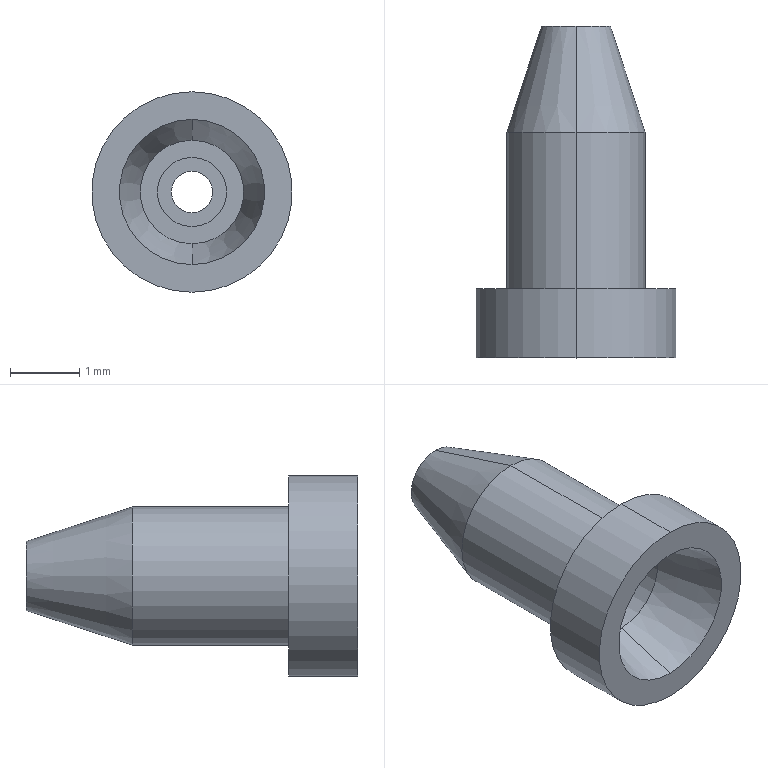Part | SolidWorks | features ICE 4, Chamfer 1, Extrusion 1, RevCut 1 | 1 solid | 19 faces | box 2.9 x 4.8 x 2.9 mm | volume 9.616 mm3 | cylinder 10 | plane 5 | cone 4 | commonest cylinder face diameters 0.6 x2 1 x2 1.5 x2 2 x2 2.9 x2
STEP:
#1=CARTESIAN_POINT('',(0.,1.,0.75));
#2=VERTEX_POINT('',#1);
#3=CARTESIAN_POINT('',(0.,1.,-0.75));
#4=VERTEX_POINT('',#3);
#5=CARTESIAN_POINT('',(0.,1.,0.));
#6=DIRECTION('',(0.,-1.,0.));
#7=DIRECTION('',(0.,0.,1.));
#8=AXIS2_PLACEMENT_3D('',#5,#6,#7);
#9=CIRCLE('',#8,0.75);
#10=EDGE_CURVE('',#2,#4,#9,.T.);
#11=ORIENTED_EDGE('',*,*,#10,.F.);
#12=CARTESIAN_POINT('',(0.,0.,1.05));
#13=VERTEX_POINT('',#12);
#14=CARTESIAN_POINT('',(0.,1.,0.75));
#15=DIRECTION('',(0.,-0.9578,0.2873));
#16=VECTOR('',#15,1000.);
#17=LINE('',#14,#16);
#18=EDGE_CURVE('',#2,#13,#17,.T.);
#19=ORIENTED_EDGE('',*,*,#18,.T.);
#20=CARTESIAN_POINT('',(0.,0.,-1.05));
#21=VERTEX_POINT('',#20);
#22=CARTESIAN_POINT('',(0.,0.,0.));
#23=DIRECTION('',(0.,1.,0.));
#24=DIRECTION('',(0.,0.,1.));
#25=AXIS2_PLACEMENT_3D('',#22,#23,#24);
#26=CIRCLE('',#25,1.05);
#27=EDGE_CURVE('',#21,#13,#26,.T.);
#28=ORIENTED_EDGE('',*,*,#27,.F.);
#29=CARTESIAN_POINT('',(0.,1.,-0.75));
#30=DIRECTION('',(0.,-0.9578,-0.2873));
#31=VECTOR('',#30,1000.);
#32=LINE('',#29,#31);
#33=EDGE_CURVE('',#4,#21,#32,.T.);
#34=ORIENTED_EDGE('',*,*,#33,.F.);
#35=EDGE_LOOP('',(#11,#19,#28,#34));
#36=FACE_OUTER_BOUND('',#35,.T.);
#37=CARTESIAN_POINT('',(0.,1.,0.));
#38=DIRECTION('',(0.,-1.,0.));
#39=DIRECTION('',(0.,0.,-1.));
#40=AXIS2_PLACEMENT_3D('',#37,#38,#39);
#41=CONICAL_SURFACE('',#40,0.75,0.2915);
#42=ADVANCED_FACE('',(#36),#41,.F.);
#43=CARTESIAN_POINT('',(0.,1.,-1.45));
#44=VERTEX_POINT('',#43);
#45=CARTESIAN_POINT('',(0.,1.,1.45));
#46=VERTEX_POINT('',#45);
#47=CARTESIAN_POINT('',(0.,1.,0.));
#48=DIRECTION('',(0.,-1.,0.));
#49=DIRECTION('',(0.,0.,-1.));
#50=AXIS2_PLACEMENT_3D('',#47,#48,#49);
#51=CIRCLE('',#50,1.45);
#52=EDGE_CURVE('',#44,#46,#51,.T.);
#53=ORIENTED_EDGE('',*,*,#52,.T.);
#54=CARTESIAN_POINT('',(0.,0.,1.45));
#55=VERTEX_POINT('',#54);
#56=CARTESIAN_POINT('',(0.,1.,1.45));
#57=DIRECTION('',(0.,-1.,0.));
#58=VECTOR('',#57,1000.);
#59=LINE('',#56,#58);
#60=EDGE_CURVE('',#46,#55,#59,.T.);
#61=ORIENTED_EDGE('',*,*,#60,.T.);
#62=CARTESIAN_POINT('',(0.,0.,-1.45));
#63=VERTEX_POINT('',#62);
#64=CARTESIAN_POINT('',(0.,0.,0.));
#65=DIRECTION('',(0.,-1.,0.));
#66=DIRECTION('',(0.,0.,-1.));
#67=AXIS2_PLACEMENT_3D('',#64,#65,#66);
#68=CIRCLE('',#67,1.45);
#69=EDGE_CURVE('',#63,#55,#68,.T.);
#70=ORIENTED_EDGE('',*,*,#69,.F.);
#71=CARTESIAN_POINT('',(0.,1.,-1.45));
#72=DIRECTION('',(0.,-1.,0.));
#73=VECTOR('',#72,1000.);
#74=LINE('',#71,#73);
#75=EDGE_CURVE('',#44,#63,#74,.T.);
#76=ORIENTED_EDGE('',*,*,#75,.F.);
#77=EDGE_LOOP('',(#53,#61,#70,#76));
#78=FACE_OUTER_BOUND('',#77,.T.);
#79=CARTESIAN_POINT('',(0.,1.,0.));
#80=DIRECTION('',(0.,-1.,0.));
#81=DIRECTION('',(0.,0.,-1.));
#82=AXIS2_PLACEMENT_3D('',#79,#80,#81);
#83=CYLINDRICAL_SURFACE('',#82,1.45);
#84=ADVANCED_FACE('',(#78),#83,.T.);
#85=CARTESIAN_POINT('',(0.,3.6,0.5));
#86=VERTEX_POINT('',#85);
#87=CARTESIAN_POINT('',(0.,3.6,-0.5));
#88=VERTEX_POINT('',#87);
#89=CARTESIAN_POINT('',(0.,3.6,0.));
#90=DIRECTION('',(0.,-1.,0.));
#91=DIRECTION('',(0.,0.,-1.));
#92=AXIS2_PLACEMENT_3D('',#89,#90,#91);
#93=CIRCLE('',#92,0.5);
#94=EDGE_CURVE('',#86,#88,#93,.T.);
#95=ORIENTED_EDGE('',*,*,#94,.F.);
#96=CARTESIAN_POINT('',(0.,3.,0.5));
#97=VERTEX_POINT('',#96);
#98=CARTESIAN_POINT('',(0.,3.6,0.5));
#99=DIRECTION('',(0.,-1.,0.));
#100=VECTOR('',#99,1000.);
#101=LINE('',#98,#100);
#102=EDGE_CURVE('',#86,#97,#101,.T.);
#103=ORIENTED_EDGE('',*,*,#102,.T.);
#104=CARTESIAN_POINT('',(0.,3.,-0.5));
#105=VERTEX_POINT('',#104);
#106=CARTESIAN_POINT('',(0.,3.,0.));
#107=DIRECTION('',(0.,-1.,0.));
#108=DIRECTION('',(0.,0.,-1.));
#109=AXIS2_PLACEMENT_3D('',#106,#107,#108);
#110=CIRCLE('',#109,0.5);
#111=EDGE_CURVE('',#97,#105,#110,.T.);
#112=ORIENTED_EDGE('',*,*,#111,.T.);
#113=CARTESIAN_POINT('',(0.,3.6,-0.5));
#114=DIRECTION('',(0.,-1.,0.));
#115=VECTOR('',#114,1000.);
#116=LINE('',#113,#115);
#117=EDGE_CURVE('',#88,#105,#116,.T.);
#118=ORIENTED_EDGE('',*,*,#117,.F.);
#119=EDGE_LOOP('',(#95,#103,#112,#118));
#120=FACE_OUTER_BOUND('',#119,.T.);
#121=CARTESIAN_POINT('',(0.,3.6,0.));
#122=DIRECTION('',(0.,-1.,0.));
#123=DIRECTION('',(0.,0.,-1.));
#124=AXIS2_PLACEMENT_3D('',#121,#122,#123);
#125=CYLINDRICAL_SURFACE('',#124,0.5);
#126=ADVANCED_FACE('',(#120),#125,.F.);
#127=CARTESIAN_POINT('',(0.,3.,0.75));
#128=VERTEX_POINT('',#127);
#129=CARTESIAN_POINT('',(0.,3.,-0.75));
#130=VERTEX_POINT('',#129);
#131=CARTESIAN_POINT('',(0.,3.,0.));
#132=DIRECTION('',(0.,-1.,0.));
#133=DIRECTION('',(0.,0.,-1.));
#134=AXIS2_PLACEMENT_3D('',#131,#132,#133);
#135=CIRCLE('',#134,0.75);
#136=EDGE_CURVE('',#128,#130,#135,.T.);
#137=ORIENTED_EDGE('',*,*,#136,.F.);
#138=CARTESIAN_POINT('',(0.,3.,0.75));
#139=DIRECTION('',(0.,-1.,0.));
#140=VECTOR('',#139,1000.);
#141=LINE('',#138,#140);
#142=EDGE_CURVE('',#128,#2,#141,.T.);
#143=ORIENTED_EDGE('',*,*,#142,.T.);
#144=ORIENTED_EDGE('',*,*,#10,.T.);
#145=CARTESIAN_POINT('',(0.,3.,-0.75));
#146=DIRECTION('',(0.,-1.,0.));
#147=VECTOR('',#146,1000.);
#148=LINE('',#145,#147);
#149=EDGE_CURVE('',#130,#4,#148,.T.);
#150=ORIENTED_EDGE('',*,*,#149,.F.);
#151=EDGE_LOOP('',(#137,#143,#144,#150));
#152=FACE_OUTER_BOUND('',#151,.T.);
#153=CARTESIAN_POINT('',(0.,3.,0.));
#154=DIRECTION('',(0.,-1.,0.));
#155=DIRECTION('',(0.,0.,-1.));
#156=AXIS2_PLACEMENT_3D('',#153,#154,#155);
#157=CYLINDRICAL_SURFACE('',#156,0.75);
#158=ADVANCED_FACE('',(#152),#157,.F.);
#159=CARTESIAN_POINT('',(0.,4.8,-0.5));
#160=VERTEX_POINT('',#159);
#161=CARTESIAN_POINT('',(0.,4.8,0.5));
#162=VERTEX_POINT('',#161);
#163=CARTESIAN_POINT('',(0.,4.8,0.));
#164=DIRECTION('',(0.,-1.,0.));
#165=DIRECTION('',(0.,0.,-1.));
#166=AXIS2_PLACEMENT_3D('',#163,#164,#165);
#167=CIRCLE('',#166,0.5);
#168=EDGE_CURVE('',#160,#162,#167,.T.);
#169=ORIENTED_EDGE('',*,*,#168,.T.);
#170=CARTESIAN_POINT('',(0.,3.261,1.));
#171=VERTEX_POINT('',#170);
#172=CARTESIAN_POINT('',(0.,4.8,0.5));
#173=DIRECTION('',(0.,-0.9511,0.309));
#174=VECTOR('',#173,1000.);
#175=LINE('',#172,#174);
#176=EDGE_CURVE('',#162,#171,#175,.T.);
#177=ORIENTED_EDGE('',*,*,#176,.T.);
#178=CARTESIAN_POINT('',(0.,3.261,-1.));
#179=VERTEX_POINT('',#178);
#180=CARTESIAN_POINT('',(0.,3.261,0.));
#181=DIRECTION('',(0.,-1.,0.));
#182=DIRECTION('',(0.,0.,-1.));
#183=AXIS2_PLACEMENT_3D('',#180,#181,#182);
#184=CIRCLE('',#183,1.);
#185=EDGE_CURVE('',#179,#171,#184,.T.);
#186=ORIENTED_EDGE('',*,*,#185,.F.);
#187=CARTESIAN_POINT('',(0.,4.8,-0.5));
#188=DIRECTION('',(0.,-0.9511,-0.309));
#189=VECTOR('',#188,1000.);
#190=LINE('',#187,#189);
#191=EDGE_CURVE('',#160,#179,#190,.T.);
#192=ORIENTED_EDGE('',*,*,#191,.F.);
#193=EDGE_LOOP('',(#169,#177,#186,#192));
#194=FACE_OUTER_BOUND('',#193,.T.);
#195=CARTESIAN_POINT('',(0.,4.8,0.));
#196=DIRECTION('',(0.,-1.,0.));
#197=DIRECTION('',(0.,0.,-1.));
#198=AXIS2_PLACEMENT_3D('',#195,#196,#197);
#199=CONICAL_SURFACE('',#198,0.5,0.3142);
#200=ADVANCED_FACE('',(#194),#199,.T.);
#201=CARTESIAN_POINT('',(0.,3.6,-0.3));
#202=VERTEX_POINT('',#201);
#203=CARTESIAN_POINT('',(0.,3.6,0.3));
#204=VERTEX_POINT('',#203);
#205=CARTESIAN_POINT('',(0.,3.6,0.));
#206=DIRECTION('',(0.,1.,0.));
#207=DIRECTION('',(0.,0.,-1.));
#208=AXIS2_PLACEMENT_3D('',#205,#206,#207);
#209=CIRCLE('',#208,0.3);
#210=EDGE_CURVE('',#202,#204,#209,.T.);
#211=ORIENTED_EDGE('',*,*,#210,.F.);
#212=CARTESIAN_POINT('',(0.,4.8,-0.3));
#213=VERTEX_POINT('',#212);
#214=CARTESIAN_POINT('',(0.,1.8,-0.3));
#215=DIRECTION('',(0.,1.,0.));
#216=VECTOR('',#215,1000.);
#217=LINE('',#214,#216);
#218=EDGE_CURVE('',#202,#213,#217,.T.);
#219=ORIENTED_EDGE('',*,*,#218,.T.);
#220=CARTESIAN_POINT('',(0.,4.8,0.3));
#221=VERTEX_POINT('',#220);
#222=CARTESIAN_POINT('',(0.,4.8,0.));
#223=DIRECTION('',(0.,1.,0.));
#224=DIRECTION('',(0.,0.,1.));
#225=AXIS2_PLACEMENT_3D('',#222,#223,#224);
#226=CIRCLE('',#225,0.3);
#227=EDGE_CURVE('',#213,#221,#226,.T.);
#228=ORIENTED_EDGE('',*,*,#227,.T.);
#229=CARTESIAN_POINT('',(0.,1.8,0.3));
#230=DIRECTION('',(0.,1.,0.));
#231=VECTOR('',#230,1000.);
#232=LINE('',#229,#231);
#233=EDGE_CURVE('',#204,#221,#232,.T.);
#234=ORIENTED_EDGE('',*,*,#233,.F.);
#235=EDGE_LOOP('',(#211,#219,#228,#234));
#236=FACE_OUTER_BOUND('',#235,.T.);
#237=CARTESIAN_POINT('',(0.,1.8,0.));
#238=DIRECTION('',(0.,1.,0.));
#239=DIRECTION('',(0.,0.,1.));
#240=AXIS2_PLACEMENT_3D('',#237,#238,#239);
#241=CYLINDRICAL_SURFACE('',#240,0.3);
#242=ADVANCED_FACE('',(#236),#241,.F.);
#243=ORIENTED_EDGE('',*,*,#185,.T.);
#244=CARTESIAN_POINT('',(0.,1.,1.));
#245=VERTEX_POINT('',#244);
#246=CARTESIAN_POINT('',(0.,4.8,1.));
#247=DIRECTION('',(0.,-1.,0.));
#248=VECTOR('',#247,1000.);
#249=LINE('',#246,#248);
#250=EDGE_CURVE('',#171,#245,#249,.T.);
#251=ORIENTED_EDGE('',*,*,#250,.T.);
#252=CARTESIAN_POINT('',(0.,1.,-1.));
#253=VERTEX_POINT('',#252);
#254=CARTESIAN_POINT('',(0.,1.,0.));
#255=DIRECTION('',(0.,-1.,0.));
#256=DIRECTION('',(0.,0.,-1.));
#257=AXIS2_PLACEMENT_3D('',#254,#255,#256);
#258=CIRCLE('',#257,1.);
#259=EDGE_CURVE('',#253,#245,#258,.T.);
#260=ORIENTED_EDGE('',*,*,#259,.F.);
#261=CARTESIAN_POINT('',(0.,4.8,-1.));
#262=DIRECTION('',(0.,-1.,0.));
#263=VECTOR('',#262,1000.);
#264=LINE('',#261,#263);
#265=EDGE_CURVE('',#179,#253,#264,.T.);
#266=ORIENTED_EDGE('',*,*,#265,.F.);
#267=EDGE_LOOP('',(#243,#251,#260,#266));
#268=FACE_OUTER_BOUND('',#267,.T.);
#269=CARTESIAN_POINT('',(0.,4.8,0.));
#270=DIRECTION('',(0.,-1.,0.));
#271=DIRECTION('',(0.,0.,-1.));
#272=AXIS2_PLACEMENT_3D('',#269,#270,#271);
#273=CYLINDRICAL_SURFACE('',#272,1.);
#274=ADVANCED_FACE('',(#268),#273,.T.);
#275=ORIENTED_EDGE('',*,*,#250,.F.);
#276=CARTESIAN_POINT('',(0.,3.261,0.));
#277=DIRECTION('',(0.,-1.,0.));
#278=DIRECTION('',(0.,0.,-1.));
#279=AXIS2_PLACEMENT_3D('',#276,#277,#278);
#280=CIRCLE('',#279,1.);
#281=EDGE_CURVE('',#171,#179,#280,.T.);
#282=ORIENTED_EDGE('',*,*,#281,.T.);
#283=ORIENTED_EDGE('',*,*,#265,.T.);
#284=CARTESIAN_POINT('',(0.,1.,0.));
#285=DIRECTION('',(0.,-1.,0.));
#286=DIRECTION('',(0.,0.,-1.));
#287=AXIS2_PLACEMENT_3D('',#284,#285,#286);
#288=CIRCLE('',#287,1.);
#289=EDGE_CURVE('',#245,#253,#288,.T.);
#290=ORIENTED_EDGE('',*,*,#289,.F.);
#291=EDGE_LOOP('',(#275,#282,#283,#290));
#292=FACE_OUTER_BOUND('',#291,.T.);
#293=CARTESIAN_POINT('',(0.,4.8,0.));
#294=DIRECTION('',(0.,-1.,0.));
#295=DIRECTION('',(0.,0.,-1.));
#296=AXIS2_PLACEMENT_3D('',#293,#294,#295);
#297=CYLINDRICAL_SURFACE('',#296,1.);
#298=ADVANCED_FACE('',(#292),#297,.T.);
#299=ORIENTED_EDGE('',*,*,#218,.F.);
#300=CARTESIAN_POINT('',(0.,3.6,0.));
#301=DIRECTION('',(0.,1.,0.));
#302=DIRECTION('',(0.,0.,-1.));
#303=AXIS2_PLACEMENT_3D('',#300,#301,#302);
#304=CIRCLE('',#303,0.3);
#305=EDGE_CURVE('',#204,#202,#304,.T.);
#306=ORIENTED_EDGE('',*,*,#305,.F.);
#307=ORIENTED_EDGE('',*,*,#233,.T.);
#308=CARTESIAN_POINT('',(0.,4.8,0.));
#309=DIRECTION('',(0.,1.,0.));
#310=DIRECTION('',(0.,0.,1.));
#311=AXIS2_PLACEMENT_3D('',#308,#309,#310);
#312=CIRCLE('',#311,0.3);
#313=EDGE_CURVE('',#221,#213,#312,.T.);
#314=ORIENTED_EDGE('',*,*,#313,.T.);
#315=EDGE_LOOP('',(#299,#306,#307,#314));
#316=FACE_OUTER_BOUND('',#315,.T.);
#317=CARTESIAN_POINT('',(0.,1.8,0.));
#318=DIRECTION('',(0.,1.,0.));
#319=DIRECTION('',(0.,0.,1.));
#320=AXIS2_PLACEMENT_3D('',#317,#318,#319);
#321=CYLINDRICAL_SURFACE('',#320,0.3);
#322=ADVANCED_FACE('',(#316),#321,.F.);
#323=ORIENTED_EDGE('',*,*,#27,.T.);
#324=CARTESIAN_POINT('',(0.,0.,0.));
#325=DIRECTION('',(0.,1.,0.));
#326=DIRECTION('',(0.,0.,1.));
#327=AXIS2_PLACEMENT_3D('',#324,#325,#326);
#328=CIRCLE('',#327,1.05);
#329=EDGE_CURVE('',#13,#21,#328,.T.);
#330=ORIENTED_EDGE('',*,*,#329,.T.);
#331=EDGE_LOOP('',(#323,#330));
#332=FACE_BOUND('',#331,.T.);
#333=ORIENTED_EDGE('',*,*,#69,.T.);
#334=CARTESIAN_POINT('',(0.,0.,0.));
#335=DIRECTION('',(0.,-1.,0.));
#336=DIRECTION('',(0.,0.,-1.));
#337=AXIS2_PLACEMENT_3D('',#334,#335,#336);
#338=CIRCLE('',#337,1.45);
#339=EDGE_CURVE('',#55,#63,#338,.T.);
#340=ORIENTED_EDGE('',*,*,#339,.T.);
#341=EDGE_LOOP('',(#333,#340));
#342=FACE_OUTER_BOUND('',#341,.T.);
#343=CARTESIAN_POINT('',(0.,0.,0.));
#344=DIRECTION('',(0.,1.,0.));
#345=DIRECTION('',(0.,0.,1.));
#346=AXIS2_PLACEMENT_3D('',#343,#344,#345);
#347=PLANE('',#346);
#348=ADVANCED_FACE('',(#332,#342),#347,.F.);
#349=ORIENTED_EDGE('',*,*,#176,.F.);
#350=CARTESIAN_POINT('',(0.,4.8,0.));
#351=DIRECTION('',(0.,-1.,0.));
#352=DIRECTION('',(0.,0.,-1.));
#353=AXIS2_PLACEMENT_3D('',#350,#351,#352);
#354=CIRCLE('',#353,0.5);
#355=EDGE_CURVE('',#162,#160,#354,.T.);
#356=ORIENTED_EDGE('',*,*,#355,.T.);
#357=ORIENTED_EDGE('',*,*,#191,.T.);
#358=ORIENTED_EDGE('',*,*,#281,.F.);
#359=EDGE_LOOP('',(#349,#356,#357,#358));
#360=FACE_OUTER_BOUND('',#359,.T.);
#361=CARTESIAN_POINT('',(0.,4.8,0.));
#362=DIRECTION('',(0.,-1.,0.));
#363=DIRECTION('',(0.,0.,-1.));
#364=AXIS2_PLACEMENT_3D('',#361,#362,#363);
#365=CONICAL_SURFACE('',#364,0.5,0.3142);
#366=ADVANCED_FACE('',(#360),#365,.T.);
#367=ORIENTED_EDGE('',*,*,#313,.F.);
#368=ORIENTED_EDGE('',*,*,#227,.F.);
#369=EDGE_LOOP('',(#367,#368));
#370=FACE_BOUND('',#369,.T.);
#371=ORIENTED_EDGE('',*,*,#168,.F.);
#372=ORIENTED_EDGE('',*,*,#355,.F.);
#373=EDGE_LOOP('',(#371,#372));
#374=FACE_OUTER_BOUND('',#373,.T.);
#375=CARTESIAN_POINT('',(0.,4.8,0.));
#376=DIRECTION('',(0.,1.,0.));
#377=DIRECTION('',(0.,0.,1.));
#378=AXIS2_PLACEMENT_3D('',#375,#376,#377);
#379=PLANE('',#378);
#380=ADVANCED_FACE('',(#370,#374),#379,.T.);
#381=ORIENTED_EDGE('',*,*,#142,.F.);
#382=CARTESIAN_POINT('',(0.,3.,0.));
#383=DIRECTION('',(0.,-1.,0.));
#384=DIRECTION('',(0.,0.,-1.));
#385=AXIS2_PLACEMENT_3D('',#382,#383,#384);
#386=CIRCLE('',#385,0.75);
#387=EDGE_CURVE('',#130,#128,#386,.T.);
#388=ORIENTED_EDGE('',*,*,#387,.F.);
#389=ORIENTED_EDGE('',*,*,#149,.T.);
#390=CARTESIAN_POINT('',(0.,1.,0.));
#391=DIRECTION('',(0.,-1.,0.));
#392=DIRECTION('',(0.,0.,1.));
#393=AXIS2_PLACEMENT_3D('',#390,#391,#392);
#394=CIRCLE('',#393,0.75);
#395=EDGE_CURVE('',#4,#2,#394,.T.);
#396=ORIENTED_EDGE('',*,*,#395,.T.);
#397=EDGE_LOOP('',(#381,#388,#389,#396));
#398=FACE_OUTER_BOUND('',#397,.T.);
#399=CARTESIAN_POINT('',(0.,3.,0.));
#400=DIRECTION('',(0.,-1.,0.));
#401=DIRECTION('',(0.,0.,-1.));
#402=AXIS2_PLACEMENT_3D('',#399,#400,#401);
#403=CYLINDRICAL_SURFACE('',#402,0.75);
#404=ADVANCED_FACE('',(#398),#403,.F.);
#405=CARTESIAN_POINT('',(0.,3.,0.));
#406=DIRECTION('',(0.,-1.,0.));
#407=DIRECTION('',(0.,0.,-1.));
#408=AXIS2_PLACEMENT_3D('',#405,#406,#407);
#409=CIRCLE('',#408,0.5);
#410=EDGE_CURVE('',#105,#97,#409,.T.);
#411=ORIENTED_EDGE('',*,*,#410,.F.);
#412=ORIENTED_EDGE('',*,*,#111,.F.);
#413=EDGE_LOOP('',(#411,#412));
#414=FACE_BOUND('',#413,.T.);
#415=ORIENTED_EDGE('',*,*,#387,.T.);
#416=ORIENTED_EDGE('',*,*,#136,.T.);
#417=EDGE_LOOP('',(#415,#416));
#418=FACE_OUTER_BOUND('',#417,.T.);
#419=CARTESIAN_POINT('',(0.,3.,0.));
#420=DIRECTION('',(0.,-1.,0.));
#421=DIRECTION('',(0.,0.,-1.));
#422=AXIS2_PLACEMENT_3D('',#419,#420,#421);
#423=PLANE('',#422);
#424=ADVANCED_FACE('',(#414,#418),#423,.T.);
#425=CARTESIAN_POINT('',(0.,3.6,0.));
#426=DIRECTION('',(0.,-1.,0.));
#427=DIRECTION('',(0.,0.,-1.));
#428=AXIS2_PLACEMENT_3D('',#425,#426,#427);
#429=CIRCLE('',#428,0.5);
#430=EDGE_CURVE('',#88,#86,#429,.T.);
#431=ORIENTED_EDGE('',*,*,#430,.T.);
#432=ORIENTED_EDGE('',*,*,#94,.T.);
#433=EDGE_LOOP('',(#431,#432));
#434=FACE_OUTER_BOUND('',#433,.T.);
#435=ORIENTED_EDGE('',*,*,#305,.T.);
#436=ORIENTED_EDGE('',*,*,#210,.T.);
#437=EDGE_LOOP('',(#435,#436));
#438=FACE_BOUND('',#437,.T.);
#439=CARTESIAN_POINT('',(0.,3.6,0.));
#440=DIRECTION('',(0.,-1.,0.));
#441=DIRECTION('',(0.,0.,-1.));
#442=AXIS2_PLACEMENT_3D('',#439,#440,#441);
#443=PLANE('',#442);
#444=ADVANCED_FACE('',(#434,#438),#443,.T.);
#445=ORIENTED_EDGE('',*,*,#102,.F.);
#446=ORIENTED_EDGE('',*,*,#430,.F.);
#447=ORIENTED_EDGE('',*,*,#117,.T.);
#448=ORIENTED_EDGE('',*,*,#410,.T.);
#449=EDGE_LOOP('',(#445,#446,#447,#448));
#450=FACE_OUTER_BOUND('',#449,.T.);
#451=CARTESIAN_POINT('',(0.,3.6,0.));
#452=DIRECTION('',(0.,-1.,0.));
#453=DIRECTION('',(0.,0.,-1.));
#454=AXIS2_PLACEMENT_3D('',#451,#452,#453);
#455=CYLINDRICAL_SURFACE('',#454,0.5);
#456=ADVANCED_FACE('',(#450),#455,.F.);
#457=ORIENTED_EDGE('',*,*,#60,.F.);
#458=CARTESIAN_POINT('',(0.,1.,0.));
#459=DIRECTION('',(0.,-1.,0.));
#460=DIRECTION('',(0.,0.,-1.));
#461=AXIS2_PLACEMENT_3D('',#458,#459,#460);
#462=CIRCLE('',#461,1.45);
#463=EDGE_CURVE('',#46,#44,#462,.T.);
#464=ORIENTED_EDGE('',*,*,#463,.T.);
#465=ORIENTED_EDGE('',*,*,#75,.T.);
#466=ORIENTED_EDGE('',*,*,#339,.F.);
#467=EDGE_LOOP('',(#457,#464,#465,#466));
#468=FACE_OUTER_BOUND('',#467,.T.);
#469=CARTESIAN_POINT('',(0.,1.,0.));
#470=DIRECTION('',(0.,-1.,0.));
#471=DIRECTION('',(0.,0.,-1.));
#472=AXIS2_PLACEMENT_3D('',#469,#470,#471);
#473=CYLINDRICAL_SURFACE('',#472,1.45);
#474=ADVANCED_FACE('',(#468),#473,.T.);
#475=ORIENTED_EDGE('',*,*,#259,.T.);
#476=ORIENTED_EDGE('',*,*,#289,.T.);
#477=EDGE_LOOP('',(#475,#476));
#478=FACE_BOUND('',#477,.T.);
#479=ORIENTED_EDGE('',*,*,#52,.F.);
#480=ORIENTED_EDGE('',*,*,#463,.F.);
#481=EDGE_LOOP('',(#479,#480));
#482=FACE_OUTER_BOUND('',#481,.T.);
#483=CARTESIAN_POINT('',(0.,1.,0.));
#484=DIRECTION('',(0.,-1.,0.));
#485=DIRECTION('',(0.,0.,-1.));
#486=AXIS2_PLACEMENT_3D('',#483,#484,#485);
#487=PLANE('',#486);
#488=ADVANCED_FACE('',(#478,#482),#487,.F.);
#489=ORIENTED_EDGE('',*,*,#18,.F.);
#490=ORIENTED_EDGE('',*,*,#395,.F.);
#491=ORIENTED_EDGE('',*,*,#33,.T.);
#492=ORIENTED_EDGE('',*,*,#329,.F.);
#493=EDGE_LOOP('',(#489,#490,#491,#492));
#494=FACE_OUTER_BOUND('',#493,.T.);
#495=CARTESIAN_POINT('',(0.,1.,0.));
#496=DIRECTION('',(0.,-1.,0.));
#497=DIRECTION('',(0.,0.,-1.));
#498=AXIS2_PLACEMENT_3D('',#495,#496,#497);
#499=CONICAL_SURFACE('',#498,0.75,0.2915);
#500=ADVANCED_FACE('',(#494),#499,.F.);
#501=CLOSED_SHELL('',(#42,#84,#126,#158,#200,#242,#274,#298,#322,#348,#366,#380,#404,#424,#444,#456,#474,#488,#500));
#502=MANIFOLD_SOLID_BREP('',#501);
#503=CARTESIAN_POINT('',(0.,0.,0.));
#504=DIRECTION('',(0.,0.,1.));
#505=DIRECTION('',(1.,0.,0.));
#506=AXIS2_PLACEMENT_3D('',#503,#504,#505);
#507=(LENGTH_UNIT()NAMED_UNIT(*)SI_UNIT(.MILLI.,.METRE.));
#508=UNCERTAINTY_MEASURE_WITH_UNIT(LENGTH_MEASURE(0.00001),#507,'','');
#509=(NAMED_UNIT(*)PLANE_ANGLE_UNIT()SI_UNIT($,.RADIAN.));
#510=(NAMED_UNIT(*)SI_UNIT($,.STERADIAN.)SOLID_ANGLE_UNIT());
#511=(GEOMETRIC_REPRESENTATION_CONTEXT(3)GLOBAL_UNCERTAINTY_ASSIGNED_CONTEXT((#508))GLOBAL_UNIT_ASSIGNED_CONTEXT((#507,#509,#510))REPRESENTATION_CONTEXT('',''));
#512=ADVANCED_BREP_SHAPE_REPRESENTATION('',(#502,#506),#511);